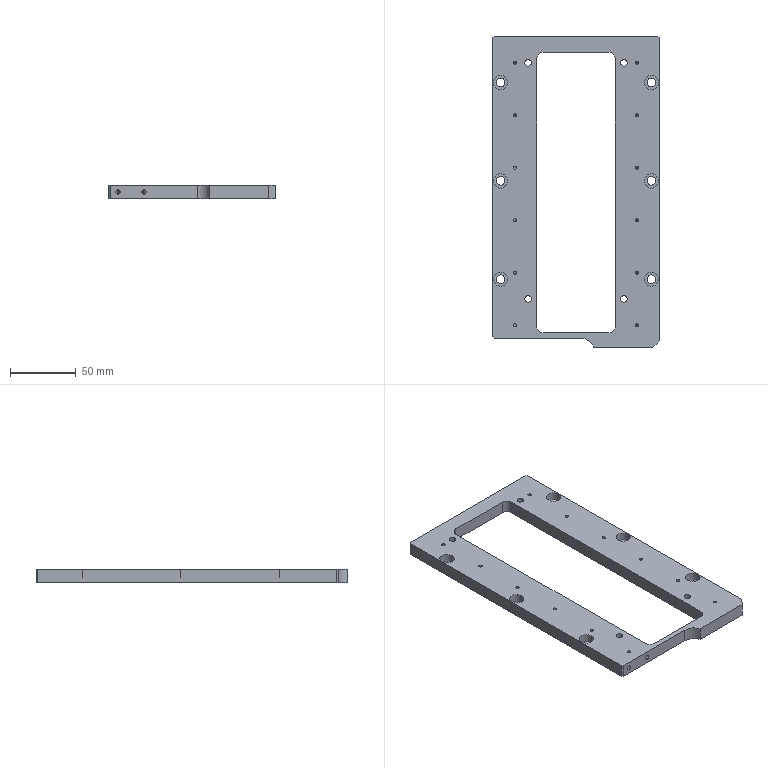Part | STEP file | 11-FG-B01811 | 1 solid | 122 faces | box 127 x 237 x 10 mm | volume 161294 mm3 | cylinder 69 | cone 32 | plane 21 | commonest cylinder face diameters 2.5 x24 6.6 x12 11 x12 3.3 x8 5 x8 10 x4